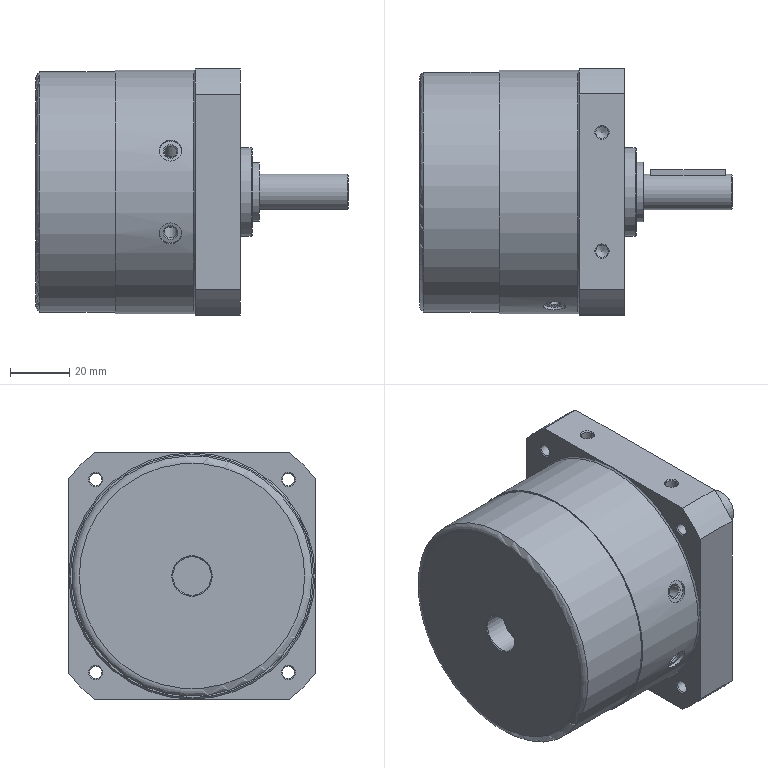Part | STEP file | 1 solid | 81 faces | box 105.5 x 83.2 x 83.2 mm | volume 387227 mm3 | plane 29 | cone 28 | cylinder 23 | torus 1 | commonest cylinder face diameters 4.134 x10 106 x4 7.5 x2 3.242 x1 12 x1 13 x1